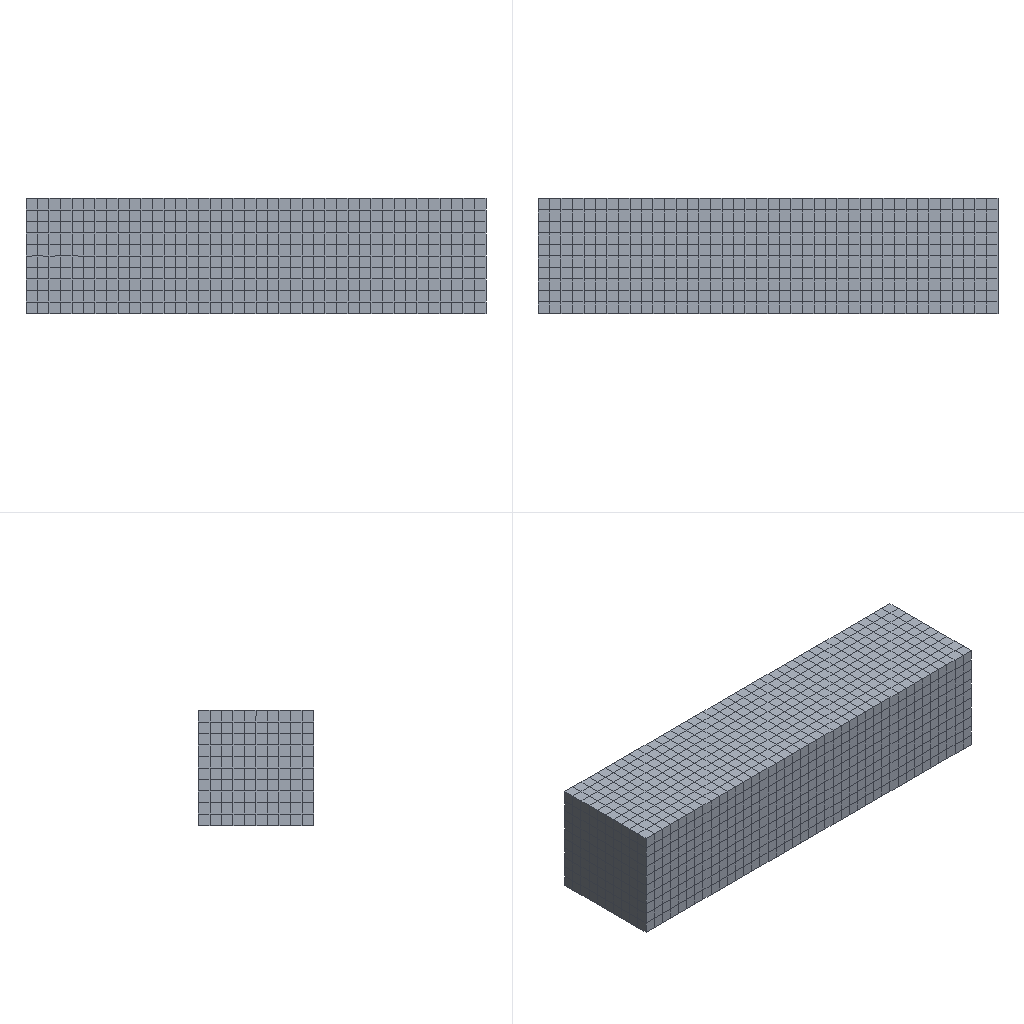Simulation study | ansys workbench
Set-up summary:
category,name,step,type,value,unit,region
solver,ansys_workbench
units,mm-N-s-tonne (MPa),,stated,"/units,MPA"
analysis,LS1,,modal,method=lanb; n_modes=6
load_step,LS1,LS1,modal
mesh,nodes,,,18822
mesh,elements,,,4000
element_type,SOLID186,,,4000
material,Beam,,E,208000,tonne s^-2 mm^-1
material,Beam,,nu,0.3
material,Beam,,density,7.85e-09,tonne mm^-3
Ansys APDL input file, long lists of numbers shortened:
/batch
/config,noeldb,1     ! force off writing results to database
*get,_wallstrt,active,,time,wall
! ANSYS input file written by Workbench version 2021 R1
! File used for geometry attach:
/title,________--__ (G5)
! ****** Begin Custom Load Command Snippet ******
/COM, ACT Extensions:
/COM,     LSDYNA, 2021.1
/COM,
! ****** End   Custom Load Command Snippet ******
*DIM,_wb_ProjectScratch_dir,string,248
_wb_ProjectScratch_dir(1) = ''
*DIM,_wb_SolverFiles_dir,string,248
_wb_SolverFiles_dir(1) = ''
*DIM,_wb_userfiles_dir,string,248
_wb_userfiles_dir(1) = ''
/com,--- Data in consistent NMM units. See Solving Units in the help system for more information.
/units,MPA
/nopr
/wb,file,start              !  signify a WB generated input file
/prep7
! Turn off shape checking because checks already performed inside WB mesher.
! See help system for more information.
SHPP,OFF,,NOWARN
/nolist
etcon,set             ! allow ANSYS to choose best KEYOP's for 180x elements, resets any applicable keyopt to MAPDL defaults
/com,*********** Nodes for the whole assembly ***********
nblock,3,,20703
(1i9,3e20.9e3)
        1     2.000000000E+00    -8.000000000E+00     8.000000000E+00
! (18820 more lines like these left out)
-1
/com,*********** Nodes for all Remote Points ***********
nblock,3
(1i9,3e20.9e3)
    18822     8.000000000E+01     0.000000000E+00     0.000000000E+00
-1
/wb,elem,start            !  set before creation of elements
/com,*********** Elements for Body 1 "___-FreeParts|____-____1" ***********
et,1,186
keyo,1,2,1          ! set full integration on SOLID186
eblock,19,solid,,4000
(19i9)
        1        1        1        1        0        0        0        0       20        0        1        1     4684     4763     4872     3510     4761     4762     4953
! (7999 more lines like these left out)
-1
/wb,elem,end               !  done creating elements
/com,*********** Send User Defined Coordinate System(s) ***********
csys,0
toffst,273.15,  ! Temperature offset from absolute zero
/com,*********** Set Reference Temperature ***********
tref,22.
/wb,mat,start              !  starting to send materials
/com,*********** Send Materials ***********
MP,EX,1,208000,	! tonne s^-2 mm^-1
MP,NUXY,1,0.3,
MP,DENS,1,7.85e-09,	! tonne mm^-3
/wb,mat,end                !  done sending materials
!************************* Model Summary ********************
!___-FreeParts|____-____1,	Beam,	matid,	1
!************************* End Model Summary ********************
! get the diagonal of the bounding box. Needed later for other things
*get,_xmin,node,,mnloc,x
*get,_ymin,node,,mnloc,y
*get,_zmin,node,,mnloc,z
*get,_xmax,node,,mxloc,x
*get,_ymax,node,,mxloc,y
*get,_zmax,node,,mxloc,z
_ASMDIAG=(_xmax-_xmin)*(_xmax-_xmin)+(_ymax-_ymin)*(_ymax-_ymin)+(_zmax-_zmin)*(_zmax-_zmin)
_ASMDIAG=SQRT(_ASMDIAG)
/wb,contact,start          !  starting to send contact
/wb,contact,end            !  done creating contacts
/golist
/wb,load,start             !  starting to send loads
/gst,on,on
fini
*get,_numnode,node,0,count
*get,_numelem,elem,0,count
*get, _MAXELEMNUM, elem, 0, NUM, MAX
*get, _MAXNODENUM, node, 0, NUM, MAX
*get, _MAXELEMTYPE, etyp, 0, NUM, MAX
*get, _MAXREALCONST, real, 0, NUM, MAX
/go
/wb,load,end               !  done creating loads
/com,--- Number of total nodes = %_numnode%
/com,--- Number of contact elements = 0
/com,--- Number of spring elements = 0
/com,--- Number of bearing elements = 0
/com,--- Number of solid elements = 4000
/com,--- Number of condensed parts = 0
/com,--- Number of total elements = %_numelem%
*get,_wallbsol,active,,time,wall
/solu
antype,2                   ! modal analysis
_thickRatio=  1     ! Ratio of thick parts in the model
modopt,lanb,6
outres,erase
outres,all,none
outres,nsol,all
outres,etmp,all
mxpand                    ! default expand in case of complex solution
dmpopt,esav,no
dmpopt,emat,no
dmpopt,full,no
! *********** WB SOLVE COMMAND ***********
! check interactive state
*get,ANSINTER_,active,,int
*if,ANSINTER_,ne,0,then
/eof
*endif
solve
/com *************** Write FE CONNECTORS *********
CEWRITE,file,ce,,INTE
*get,_nmodalsolproc,active,0,numcpu
fini
/nopr
*get,_numnode,node,0,count
*get,_numelem,elem,0,count
*get, _MAXELEMNUM, elem, 0, NUM, MAX
*get, _MAXNODENUM, node, 0, NUM, MAX,,,INTERNAL
*get, _MAXELEMTYPE, etyp, 0, NUM, MAX
*get, _MAXREALCONST, real, 0, NUM, MAX
/gopr
*get,_wallasol,active,,time,wall
/post1
/nopr
*dim,_direction,CHAR,6,1
_direction(1) = 'X'
_direction(2) = 'Y'
_direction(3) = 'Z'
_direction(4) = 'ROTX'
_direction(5) = 'ROTY'
_direction(6) = 'ROTZ'
*get,_lastLS,active,0,set,LSTP
*get,_beginset,active,0,set,nset,first,_lastLS
*get,_endset,active,0,set,nset,last,_lastLS
_nummodes = 0
*if,_endset,gt,0,then
_nummodes = _endset - _beginset + 1
*endif
*do,i_mode,1,_nummodes
   *do,j_component,1,6
			*get,PFACT_%i_mode%_%j_component%,MODE,%i_mode%,PFACT,,DIREC,_direction(%j_component%)
   *enddo
*enddo
*dim,_tmdirection,CHAR,6,1
_tmdirection(1) = 'X'
_tmdirection(2) = 'Y'
_tmdirection(3) = 'Z'
_tmdirection(4) = 'X'
_tmdirection(5) = 'Y'
_tmdirection(6) = 'Z'
*do,j_component,1,6
    *if,j_component,gt,3,then
        *get,TOTALMASS_%j_component%,ELEM,0,IOR,_tmdirection(%j_component%)
    *else
        *get,TOTALMASS_%j_component%,ELEM,0,MTOT,_tmdirection(%j_component%)
    *endif
*enddo
/gopr
xmlo,ENCODING,ISO-8859-1
xmlo,parm
/xml,parm,xml
fini
/gopr
*get,_walldone,active,,time,wall
_preptime=(_wallbsol-_wallstrt)*3600
_solvtime=(_wallasol-_wallbsol)*3600
_posttime=(_walldone-_wallasol)*3600
_totaltim=(_walldone-_wallstrt)*3600
*get,_dlbratio,active,0,solu,dlbr
*get,_combtime,active,0,solu,comb
/com,--- Total number of nodes = %_numnode%
/com,--- Total number of elements = %_numelem%
/com,--- Element load balance ratio = %_dlbratio%
/com,--- Time to combine distributed files = %_combtime%
/wb,file,end               ! done with WB generated input
Results summary:
result,analyses[0].index,,,1
result,analyses[0].system,,,SYS-6
result,analyses[0].deck,,,deck.dat
result,analyses[0].solve_status,,,completed
result,analyses[0].analysis_type,,,modal
result,analyses[0].physics,,,mechanical
result,analyses[0].unit_system,,,"NMM: mm, ton, N, s, mV, mA, degC"
result,analyses[0].n_sets,,,6
result,analyses[0].modal_frequencies_hz[1],,,0
result,analyses[0].modal_frequencies_hz[2],,,0
result,analyses[0].modal_frequencies_hz[3],,,0
result,analyses[0].modal_frequencies_hz[4],,,0.00614
result,analyses[0].modal_frequencies_hz[5],,,0.01215
result,analyses[0].modal_frequencies_hz[6],,,0.0304
result,geometry_export[0][0],,,.step
result,geometry_export[0][1],,,ok
result,geometry_export[0][2],,,1